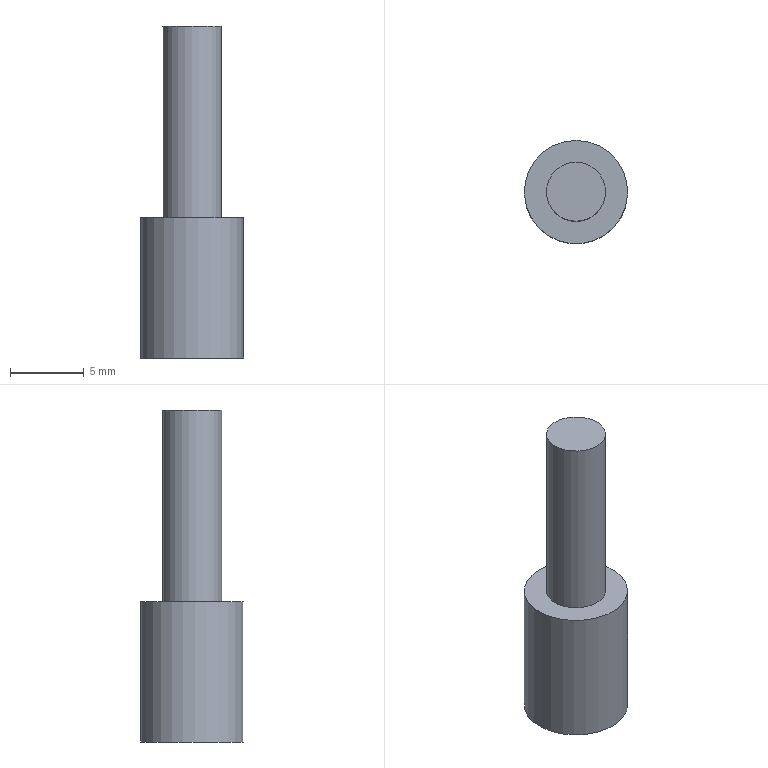Part | STEP file | 1-54.3 | 1 solid | 5 faces | box 7 x 7 x 22.5 mm | volume 528.966 mm3 | plane 3 | cylinder 2 | commonest cylinder face diameters 4 x1 7 x1
STEP:
#1=CARTESIAN_POINT('',(0.,0.,0.));
#2=DIRECTION('',(0.,0.,1.));
#3=DIRECTION('',(1.,0.,0.));
#4=AXIS2_PLACEMENT_3D('',#1,#2,#3);
#5=CARTESIAN_POINT('',(0.,3.5,-9.5));
#6=VERTEX_POINT('',#5);
#7=CARTESIAN_POINT('',(0.,0.,-9.5));
#8=DIRECTION('',(0.,0.,1.));
#9=DIRECTION('',(0.,1.,0.));
#10=AXIS2_PLACEMENT_3D('',#7,#8,#9);
#11=CIRCLE('',#10,3.5);
#12=CARTESIAN_POINT('',(0.,-0.9378,-9.5));
#13=DIRECTION('',(0.,0.,1.));
#14=DIRECTION('',(1.,0.,0.));
#15=AXIS2_PLACEMENT_3D('',#12,#13,#14);
#16=PLANE('',#15);
#17=CARTESIAN_POINT('',(0.,0.9378));
#18=DIRECTION('',(0.,1.));
#19=AXIS2_PLACEMENT_2D('',#17,#18);
#20=CIRCLE('',#19,3.5);
#21=(GEOMETRIC_REPRESENTATION_CONTEXT(2)PARAMETRIC_REPRESENTATION_CONTEXT()REPRESENTATION_CONTEXT('',''));
#22=DEFINITIONAL_REPRESENTATION('',(#20),#21);
#23=PCURVE('',#16,#22);
#24=CARTESIAN_POINT('',(0.,0.,0.));
#25=DIRECTION('',(0.,0.,-1.));
#26=DIRECTION('',(0.,1.,0.));
#27=AXIS2_PLACEMENT_3D('',#24,#25,#26);
#28=CYLINDRICAL_SURFACE('',#27,3.5);
#29=CARTESIAN_POINT('',(6.283,9.5));
#30=DIRECTION('',(-1.,0.));
#31=VECTOR('',#30,1.);
#32=LINE('',#29,#31);
#33=(GEOMETRIC_REPRESENTATION_CONTEXT(2)PARAMETRIC_REPRESENTATION_CONTEXT()REPRESENTATION_CONTEXT('',''));
#34=DEFINITIONAL_REPRESENTATION('',(#32),#33);
#35=PCURVE('',#28,#34);
#36=SURFACE_CURVE('',#11,(#23,#35),.PCURVE_S1.);
#37=EDGE_CURVE('',#6,#6,#36,.T.);
#38=ORIENTED_EDGE('',*,*,#37,.T.);
#39=EDGE_LOOP('',(#38));
#40=FACE_BOUND('',#39,.F.);
#41=ADVANCED_FACE('',(#40),#16,.F.);
#42=CARTESIAN_POINT('',(0.,3.5,0.));
#43=VERTEX_POINT('',#42);
#44=CARTESIAN_POINT('',(0.,3.5,0.));
#45=DIRECTION('',(0.,0.,-1.));
#46=VECTOR('',#45,1.);
#47=LINE('',#44,#46);
#48=CARTESIAN_POINT('',(6.283,0.));
#49=DIRECTION('',(0.,1.));
#50=VECTOR('',#49,1.);
#51=LINE('',#48,#50);
#52=(GEOMETRIC_REPRESENTATION_CONTEXT(2)PARAMETRIC_REPRESENTATION_CONTEXT()REPRESENTATION_CONTEXT('',''));
#53=DEFINITIONAL_REPRESENTATION('',(#51),#52);
#54=PCURVE('',#28,#53);
#55=CARTESIAN_POINT('',(0.,0.));
#56=DIRECTION('',(0.,1.));
#57=VECTOR('',#56,1.);
#58=LINE('',#55,#57);
#59=(GEOMETRIC_REPRESENTATION_CONTEXT(2)PARAMETRIC_REPRESENTATION_CONTEXT()REPRESENTATION_CONTEXT('',''));
#60=DEFINITIONAL_REPRESENTATION('',(#58),#59);
#61=PCURVE('',#28,#60);
#62=SEAM_CURVE('',#47,(#54,#61),.PCURVE_S1.);
#63=EDGE_CURVE('',#43,#6,#62,.T.);
#64=ORIENTED_EDGE('',*,*,#63,.T.);
#65=ORIENTED_EDGE('',*,*,#37,.T.);
#66=ORIENTED_EDGE('',*,*,#63,.F.);
#67=CARTESIAN_POINT('',(0.,0.,0.));
#68=DIRECTION('',(0.,0.,1.));
#69=DIRECTION('',(0.,1.,0.));
#70=AXIS2_PLACEMENT_3D('',#67,#68,#69);
#71=CIRCLE('',#70,3.5);
#72=CARTESIAN_POINT('',(6.283,0.));
#73=DIRECTION('',(-1.,0.));
#74=VECTOR('',#73,1.);
#75=LINE('',#72,#74);
#76=(GEOMETRIC_REPRESENTATION_CONTEXT(2)PARAMETRIC_REPRESENTATION_CONTEXT()REPRESENTATION_CONTEXT('',''));
#77=DEFINITIONAL_REPRESENTATION('',(#75),#76);
#78=PCURVE('',#28,#77);
#79=CARTESIAN_POINT('',(0.,-0.9378,0.));
#80=DIRECTION('',(0.,0.,1.));
#81=DIRECTION('',(1.,0.,0.));
#82=AXIS2_PLACEMENT_3D('',#79,#80,#81);
#83=PLANE('',#82);
#84=CARTESIAN_POINT('',(0.,0.9378));
#85=DIRECTION('',(0.,1.));
#86=AXIS2_PLACEMENT_2D('',#84,#85);
#87=CIRCLE('',#86,3.5);
#88=(GEOMETRIC_REPRESENTATION_CONTEXT(2)PARAMETRIC_REPRESENTATION_CONTEXT()REPRESENTATION_CONTEXT('',''));
#89=DEFINITIONAL_REPRESENTATION('',(#87),#88);
#90=PCURVE('',#83,#89);
#91=SURFACE_CURVE('',#71,(#78,#90),.PCURVE_S1.);
#92=EDGE_CURVE('',#43,#43,#91,.T.);
#93=ORIENTED_EDGE('',*,*,#92,.F.);
#94=EDGE_LOOP('',(#64,#65,#66,#93));
#95=FACE_BOUND('',#94,.T.);
#96=ADVANCED_FACE('',(#95),#28,.T.);
#97=ORIENTED_EDGE('',*,*,#92,.T.);
#98=EDGE_LOOP('',(#97));
#99=FACE_BOUND('',#98,.T.);
#100=CARTESIAN_POINT('',(0.,2.,0.));
#101=VERTEX_POINT('',#100);
#102=CARTESIAN_POINT('',(0.,0.,0.));
#103=DIRECTION('',(0.,0.,1.));
#104=DIRECTION('',(0.,1.,0.));
#105=AXIS2_PLACEMENT_3D('',#102,#103,#104);
#106=CIRCLE('',#105,2.);
#107=CARTESIAN_POINT('',(0.,0.9378));
#108=DIRECTION('',(0.,1.));
#109=AXIS2_PLACEMENT_2D('',#107,#108);
#110=CIRCLE('',#109,2.);
#111=(GEOMETRIC_REPRESENTATION_CONTEXT(2)PARAMETRIC_REPRESENTATION_CONTEXT()REPRESENTATION_CONTEXT('',''));
#112=DEFINITIONAL_REPRESENTATION('',(#110),#111);
#113=PCURVE('',#83,#112);
#114=CARTESIAN_POINT('',(0.,0.,0.));
#115=DIRECTION('',(0.,0.,1.));
#116=DIRECTION('',(0.,1.,0.));
#117=AXIS2_PLACEMENT_3D('',#114,#115,#116);
#118=CYLINDRICAL_SURFACE('',#117,2.);
#119=CARTESIAN_POINT('',(0.,0.));
#120=DIRECTION('',(1.,0.));
#121=VECTOR('',#120,1.);
#122=LINE('',#119,#121);
#123=(GEOMETRIC_REPRESENTATION_CONTEXT(2)PARAMETRIC_REPRESENTATION_CONTEXT()REPRESENTATION_CONTEXT('',''));
#124=DEFINITIONAL_REPRESENTATION('',(#122),#123);
#125=PCURVE('',#118,#124);
#126=SURFACE_CURVE('',#106,(#113,#125),.PCURVE_S1.);
#127=EDGE_CURVE('',#101,#101,#126,.T.);
#128=ORIENTED_EDGE('',*,*,#127,.F.);
#129=EDGE_LOOP('',(#128));
#130=FACE_BOUND('',#129,.T.);
#131=ADVANCED_FACE('',(#99,#130),#83,.T.);
#132=ORIENTED_EDGE('',*,*,#127,.T.);
#133=CARTESIAN_POINT('',(0.,2.,13.));
#134=VERTEX_POINT('',#133);
#135=CARTESIAN_POINT('',(0.,2.,0.));
#136=DIRECTION('',(0.,0.,1.));
#137=VECTOR('',#136,1.);
#138=LINE('',#135,#137);
#139=CARTESIAN_POINT('',(6.283,0.));
#140=DIRECTION('',(0.,1.));
#141=VECTOR('',#140,1.);
#142=LINE('',#139,#141);
#143=(GEOMETRIC_REPRESENTATION_CONTEXT(2)PARAMETRIC_REPRESENTATION_CONTEXT()REPRESENTATION_CONTEXT('',''));
#144=DEFINITIONAL_REPRESENTATION('',(#142),#143);
#145=PCURVE('',#118,#144);
#146=CARTESIAN_POINT('',(0.,0.));
#147=DIRECTION('',(0.,1.));
#148=VECTOR('',#147,1.);
#149=LINE('',#146,#148);
#150=(GEOMETRIC_REPRESENTATION_CONTEXT(2)PARAMETRIC_REPRESENTATION_CONTEXT()REPRESENTATION_CONTEXT('',''));
#151=DEFINITIONAL_REPRESENTATION('',(#149),#150);
#152=PCURVE('',#118,#151);
#153=SEAM_CURVE('',#138,(#145,#152),.PCURVE_S1.);
#154=EDGE_CURVE('',#101,#134,#153,.T.);
#155=ORIENTED_EDGE('',*,*,#154,.T.);
#156=CARTESIAN_POINT('',(0.,0.,13.));
#157=DIRECTION('',(0.,0.,1.));
#158=DIRECTION('',(0.,1.,0.));
#159=AXIS2_PLACEMENT_3D('',#156,#157,#158);
#160=CIRCLE('',#159,2.);
#161=CARTESIAN_POINT('',(0.,13.));
#162=DIRECTION('',(1.,0.));
#163=VECTOR('',#162,1.);
#164=LINE('',#161,#163);
#165=(GEOMETRIC_REPRESENTATION_CONTEXT(2)PARAMETRIC_REPRESENTATION_CONTEXT()REPRESENTATION_CONTEXT('',''));
#166=DEFINITIONAL_REPRESENTATION('',(#164),#165);
#167=PCURVE('',#118,#166);
#168=CARTESIAN_POINT('',(0.,-0.5359,13.));
#169=DIRECTION('',(0.,0.,1.));
#170=DIRECTION('',(1.,0.,0.));
#171=AXIS2_PLACEMENT_3D('',#168,#169,#170);
#172=PLANE('',#171);
#173=CARTESIAN_POINT('',(0.,0.5359));
#174=DIRECTION('',(0.,1.));
#175=AXIS2_PLACEMENT_2D('',#173,#174);
#176=CIRCLE('',#175,2.);
#177=(GEOMETRIC_REPRESENTATION_CONTEXT(2)PARAMETRIC_REPRESENTATION_CONTEXT()REPRESENTATION_CONTEXT('',''));
#178=DEFINITIONAL_REPRESENTATION('',(#176),#177);
#179=PCURVE('',#172,#178);
#180=SURFACE_CURVE('',#160,(#167,#179),.PCURVE_S1.);
#181=EDGE_CURVE('',#134,#134,#180,.T.);
#182=ORIENTED_EDGE('',*,*,#181,.F.);
#183=ORIENTED_EDGE('',*,*,#154,.F.);
#184=EDGE_LOOP('',(#132,#155,#182,#183));
#185=FACE_BOUND('',#184,.T.);
#186=ADVANCED_FACE('',(#185),#118,.T.);
#187=ORIENTED_EDGE('',*,*,#181,.T.);
#188=EDGE_LOOP('',(#187));
#189=FACE_BOUND('',#188,.T.);
#190=ADVANCED_FACE('',(#189),#172,.T.);
#191=CLOSED_SHELL('',(#41,#96,#131,#186,#190));
#192=MANIFOLD_SOLID_BREP('',#191);
#193=(LENGTH_UNIT()NAMED_UNIT(*)SI_UNIT(.MILLI.,.METRE.));
#194=UNCERTAINTY_MEASURE_WITH_UNIT(LENGTH_MEASURE(0.0000001),#193,'','');
#195=(NAMED_UNIT(*)PLANE_ANGLE_UNIT()SI_UNIT($,.RADIAN.));
#196=(NAMED_UNIT(*)SI_UNIT($,.STERADIAN.)SOLID_ANGLE_UNIT());
#197=(GEOMETRIC_REPRESENTATION_CONTEXT(3)GLOBAL_UNCERTAINTY_ASSIGNED_CONTEXT((#194))GLOBAL_UNIT_ASSIGNED_CONTEXT((#193,#195,#196))REPRESENTATION_CONTEXT('',''));
#198=ADVANCED_BREP_SHAPE_REPRESENTATION('',(#4,#192),#197);